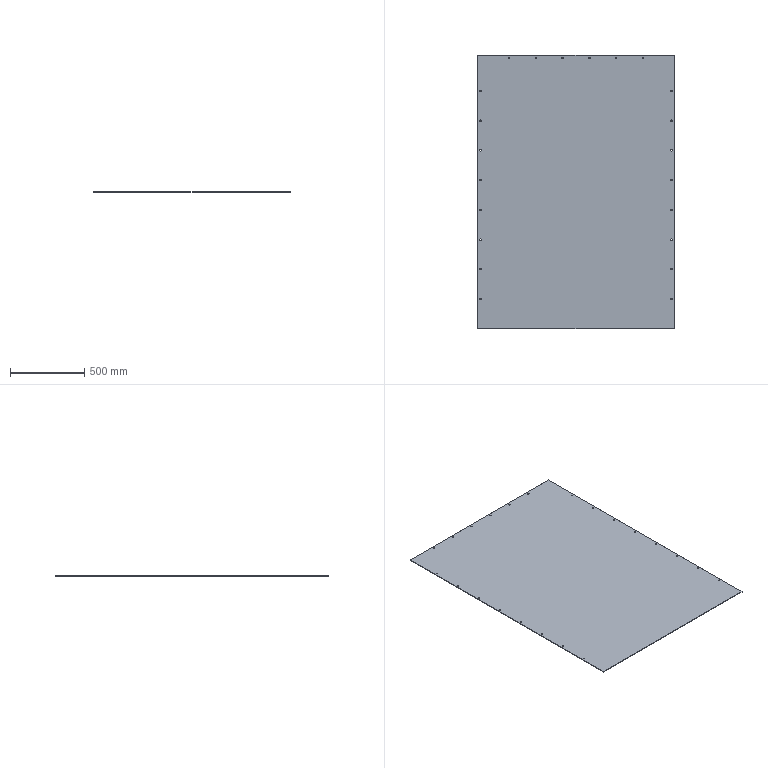Part | SolidWorks | features FlatPattern 1, SMBaseFlange 1, SheetMetal 1 | 1 solid | 50 faces | box 1320 x 1840 x 4 mm | volume 9708288 mm3 | cylinder 44 | plane 6 | commonest cylinder face diameters 10 x44